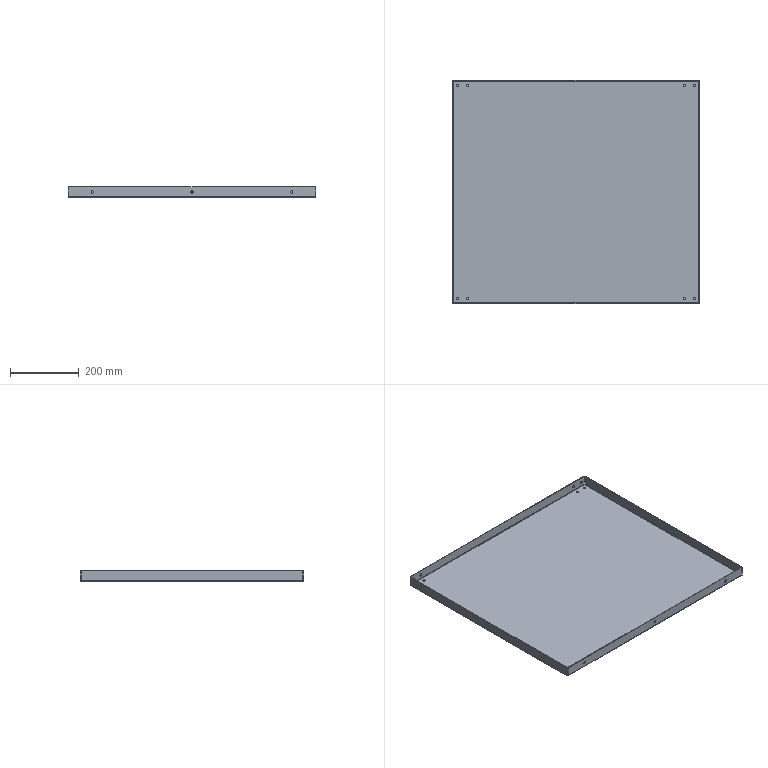Part | STEP file | Rear sheet metal | 1 solid | 68 faces | box 720 x 650 x 30 mm | volume 814414 mm3 | cylinder 38 | plane 22 | spline 8 | commonest cylinder face diameters 7 x30 2 x4 5 x4